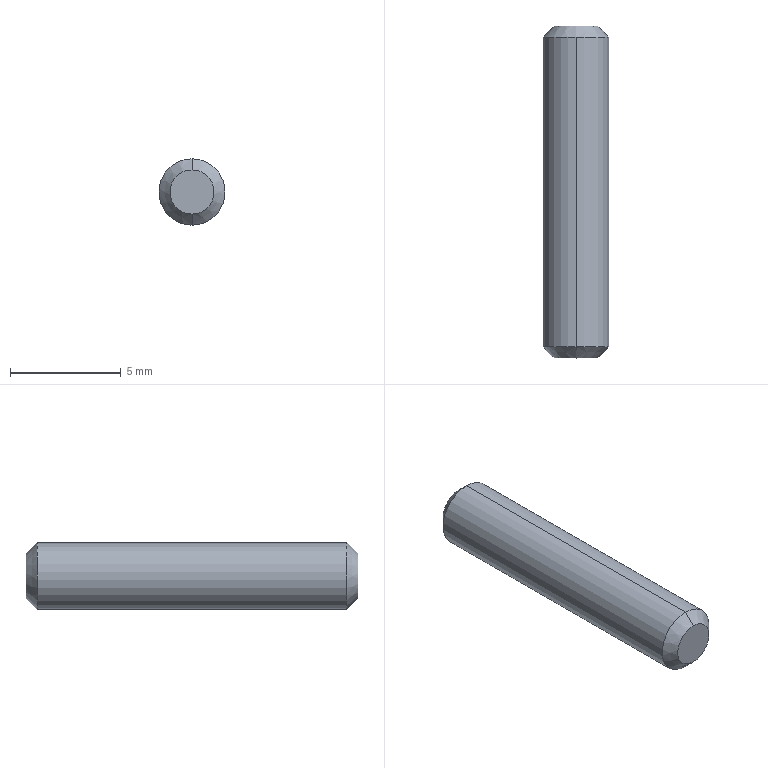Part | SolidWorks | features Chamfer 1, Extrusion 1 | 1 solid | 8 faces | box 3 x 15 x 3 mm | volume 103.934 mm3 | cone 4 | cylinder 2 | plane 2 | commonest cylinder face diameters 3 x2
STEP:
#1=CARTESIAN_POINT('',(0.,15.,1.));
#2=VERTEX_POINT('',#1);
#3=CARTESIAN_POINT('',(0.,15.,-1.));
#4=VERTEX_POINT('',#3);
#5=CARTESIAN_POINT('',(0.,15.,0.));
#6=DIRECTION('',(0.,1.,0.));
#7=DIRECTION('',(0.,0.,1.));
#8=AXIS2_PLACEMENT_3D('',#5,#6,#7);
#9=CIRCLE('',#8,1.);
#10=EDGE_CURVE('',#2,#4,#9,.T.);
#11=ORIENTED_EDGE('',*,*,#10,.F.);
#12=CARTESIAN_POINT('',(0.,14.5,1.5));
#13=VERTEX_POINT('',#12);
#14=CARTESIAN_POINT('',(0.,15.,1.));
#15=DIRECTION('',(0.,-0.7071,0.7071));
#16=VECTOR('',#15,1000.);
#17=LINE('',#14,#16);
#18=EDGE_CURVE('',#2,#13,#17,.T.);
#19=ORIENTED_EDGE('',*,*,#18,.T.);
#20=CARTESIAN_POINT('',(0.,14.5,-1.5));
#21=VERTEX_POINT('',#20);
#22=CARTESIAN_POINT('',(0.,14.5,0.));
#23=DIRECTION('',(0.,-1.,0.));
#24=DIRECTION('',(0.,0.,1.));
#25=AXIS2_PLACEMENT_3D('',#22,#23,#24);
#26=CIRCLE('',#25,1.5);
#27=EDGE_CURVE('',#21,#13,#26,.T.);
#28=ORIENTED_EDGE('',*,*,#27,.F.);
#29=CARTESIAN_POINT('',(0.,15.,-1.));
#30=DIRECTION('',(0.,-0.7071,-0.7071));
#31=VECTOR('',#30,1000.);
#32=LINE('',#29,#31);
#33=EDGE_CURVE('',#4,#21,#32,.T.);
#34=ORIENTED_EDGE('',*,*,#33,.F.);
#35=EDGE_LOOP('',(#11,#19,#28,#34));
#36=FACE_OUTER_BOUND('',#35,.T.);
#37=CARTESIAN_POINT('',(0.,15.,0.));
#38=DIRECTION('',(0.,-1.,0.));
#39=DIRECTION('',(0.,0.,-1.));
#40=AXIS2_PLACEMENT_3D('',#37,#38,#39);
#41=CONICAL_SURFACE('',#40,1.,0.7854);
#42=ADVANCED_FACE('',(#36),#41,.T.);
#43=CARTESIAN_POINT('',(0.,0.,-1.));
#44=VERTEX_POINT('',#43);
#45=CARTESIAN_POINT('',(0.,0.,1.));
#46=VERTEX_POINT('',#45);
#47=CARTESIAN_POINT('',(0.,0.,0.));
#48=DIRECTION('',(0.,-1.,0.));
#49=DIRECTION('',(0.,0.,1.));
#50=AXIS2_PLACEMENT_3D('',#47,#48,#49);
#51=CIRCLE('',#50,1.);
#52=EDGE_CURVE('',#44,#46,#51,.T.);
#53=ORIENTED_EDGE('',*,*,#52,.F.);
#54=CARTESIAN_POINT('',(0.,0.5,-1.5));
#55=VERTEX_POINT('',#54);
#56=CARTESIAN_POINT('',(0.,0.5,-1.5));
#57=DIRECTION('',(0.,0.7071,-0.7071));
#58=VECTOR('',#57,1000.);
#59=LINE('',#56,#58);
#60=EDGE_CURVE('',#44,#55,#59,.T.);
#61=ORIENTED_EDGE('',*,*,#60,.T.);
#62=CARTESIAN_POINT('',(0.,0.5,1.5));
#63=VERTEX_POINT('',#62);
#64=CARTESIAN_POINT('',(0.,0.5,0.));
#65=DIRECTION('',(0.,1.,0.));
#66=DIRECTION('',(0.,0.,1.));
#67=AXIS2_PLACEMENT_3D('',#64,#65,#66);
#68=CIRCLE('',#67,1.5);
#69=EDGE_CURVE('',#63,#55,#68,.T.);
#70=ORIENTED_EDGE('',*,*,#69,.F.);
#71=CARTESIAN_POINT('',(0.,0.5,1.5));
#72=DIRECTION('',(0.,0.7071,0.7071));
#73=VECTOR('',#72,1000.);
#74=LINE('',#71,#73);
#75=EDGE_CURVE('',#46,#63,#74,.T.);
#76=ORIENTED_EDGE('',*,*,#75,.F.);
#77=EDGE_LOOP('',(#53,#61,#70,#76));
#78=FACE_OUTER_BOUND('',#77,.T.);
#79=CARTESIAN_POINT('',(0.,0.5,0.));
#80=DIRECTION('',(0.,1.,0.));
#81=DIRECTION('',(0.,0.,1.));
#82=AXIS2_PLACEMENT_3D('',#79,#80,#81);
#83=CONICAL_SURFACE('',#82,1.5,0.7854);
#84=ADVANCED_FACE('',(#78),#83,.T.);
#85=ORIENTED_EDGE('',*,*,#27,.T.);
#86=CARTESIAN_POINT('',(0.,15.,1.5));
#87=DIRECTION('',(0.,-1.,0.));
#88=VECTOR('',#87,1000.);
#89=LINE('',#86,#88);
#90=EDGE_CURVE('',#13,#63,#89,.T.);
#91=ORIENTED_EDGE('',*,*,#90,.T.);
#92=ORIENTED_EDGE('',*,*,#69,.T.);
#93=CARTESIAN_POINT('',(0.,15.,-1.5));
#94=DIRECTION('',(0.,-1.,0.));
#95=VECTOR('',#94,1000.);
#96=LINE('',#93,#95);
#97=EDGE_CURVE('',#21,#55,#96,.T.);
#98=ORIENTED_EDGE('',*,*,#97,.F.);
#99=EDGE_LOOP('',(#85,#91,#92,#98));
#100=FACE_OUTER_BOUND('',#99,.T.);
#101=CARTESIAN_POINT('',(0.,15.,0.));
#102=DIRECTION('',(0.,-1.,0.));
#103=DIRECTION('',(0.,0.,-1.));
#104=AXIS2_PLACEMENT_3D('',#101,#102,#103);
#105=CYLINDRICAL_SURFACE('',#104,1.5);
#106=ADVANCED_FACE('',(#100),#105,.T.);
#107=ORIENTED_EDGE('',*,*,#90,.F.);
#108=CARTESIAN_POINT('',(0.,14.5,0.));
#109=DIRECTION('',(0.,-1.,0.));
#110=DIRECTION('',(0.,0.,1.));
#111=AXIS2_PLACEMENT_3D('',#108,#109,#110);
#112=CIRCLE('',#111,1.5);
#113=EDGE_CURVE('',#13,#21,#112,.T.);
#114=ORIENTED_EDGE('',*,*,#113,.T.);
#115=ORIENTED_EDGE('',*,*,#97,.T.);
#116=CARTESIAN_POINT('',(0.,0.5,0.));
#117=DIRECTION('',(0.,1.,0.));
#118=DIRECTION('',(0.,0.,1.));
#119=AXIS2_PLACEMENT_3D('',#116,#117,#118);
#120=CIRCLE('',#119,1.5);
#121=EDGE_CURVE('',#55,#63,#120,.T.);
#122=ORIENTED_EDGE('',*,*,#121,.T.);
#123=EDGE_LOOP('',(#107,#114,#115,#122));
#124=FACE_OUTER_BOUND('',#123,.T.);
#125=CARTESIAN_POINT('',(0.,15.,0.));
#126=DIRECTION('',(0.,-1.,0.));
#127=DIRECTION('',(0.,0.,-1.));
#128=AXIS2_PLACEMENT_3D('',#125,#126,#127);
#129=CYLINDRICAL_SURFACE('',#128,1.5);
#130=ADVANCED_FACE('',(#124),#129,.T.);
#131=CARTESIAN_POINT('',(0.,15.,0.));
#132=DIRECTION('',(0.,1.,0.));
#133=DIRECTION('',(0.,0.,1.));
#134=AXIS2_PLACEMENT_3D('',#131,#132,#133);
#135=CIRCLE('',#134,1.);
#136=EDGE_CURVE('',#4,#2,#135,.T.);
#137=ORIENTED_EDGE('',*,*,#136,.T.);
#138=ORIENTED_EDGE('',*,*,#10,.T.);
#139=EDGE_LOOP('',(#137,#138));
#140=FACE_OUTER_BOUND('',#139,.T.);
#141=CARTESIAN_POINT('',(0.,15.,0.));
#142=DIRECTION('',(0.,1.,0.));
#143=DIRECTION('',(0.,0.,1.));
#144=AXIS2_PLACEMENT_3D('',#141,#142,#143);
#145=PLANE('',#144);
#146=ADVANCED_FACE('',(#140),#145,.T.);
#147=CARTESIAN_POINT('',(0.,0.,0.));
#148=DIRECTION('',(0.,-1.,0.));
#149=DIRECTION('',(0.,0.,1.));
#150=AXIS2_PLACEMENT_3D('',#147,#148,#149);
#151=CIRCLE('',#150,1.);
#152=EDGE_CURVE('',#46,#44,#151,.T.);
#153=ORIENTED_EDGE('',*,*,#152,.T.);
#154=ORIENTED_EDGE('',*,*,#52,.T.);
#155=EDGE_LOOP('',(#153,#154));
#156=FACE_OUTER_BOUND('',#155,.T.);
#157=CARTESIAN_POINT('',(0.,0.,0.));
#158=DIRECTION('',(0.,1.,0.));
#159=DIRECTION('',(0.,0.,1.));
#160=AXIS2_PLACEMENT_3D('',#157,#158,#159);
#161=PLANE('',#160);
#162=ADVANCED_FACE('',(#156),#161,.F.);
#163=ORIENTED_EDGE('',*,*,#60,.F.);
#164=ORIENTED_EDGE('',*,*,#152,.F.);
#165=ORIENTED_EDGE('',*,*,#75,.T.);
#166=ORIENTED_EDGE('',*,*,#121,.F.);
#167=EDGE_LOOP('',(#163,#164,#165,#166));
#168=FACE_OUTER_BOUND('',#167,.T.);
#169=CARTESIAN_POINT('',(0.,0.5,0.));
#170=DIRECTION('',(0.,1.,0.));
#171=DIRECTION('',(0.,0.,1.));
#172=AXIS2_PLACEMENT_3D('',#169,#170,#171);
#173=CONICAL_SURFACE('',#172,1.5,0.7854);
#174=ADVANCED_FACE('',(#168),#173,.T.);
#175=ORIENTED_EDGE('',*,*,#18,.F.);
#176=ORIENTED_EDGE('',*,*,#136,.F.);
#177=ORIENTED_EDGE('',*,*,#33,.T.);
#178=ORIENTED_EDGE('',*,*,#113,.F.);
#179=EDGE_LOOP('',(#175,#176,#177,#178));
#180=FACE_OUTER_BOUND('',#179,.T.);
#181=CARTESIAN_POINT('',(0.,15.,0.));
#182=DIRECTION('',(0.,-1.,0.));
#183=DIRECTION('',(0.,0.,-1.));
#184=AXIS2_PLACEMENT_3D('',#181,#182,#183);
#185=CONICAL_SURFACE('',#184,1.,0.7854);
#186=ADVANCED_FACE('',(#180),#185,.T.);
#187=CLOSED_SHELL('',(#42,#84,#106,#130,#146,#162,#174,#186));
#188=MANIFOLD_SOLID_BREP('',#187);
#189=CARTESIAN_POINT('',(0.,0.,0.));
#190=DIRECTION('',(0.,0.,1.));
#191=DIRECTION('',(1.,0.,0.));
#192=AXIS2_PLACEMENT_3D('',#189,#190,#191);
#193=(LENGTH_UNIT()NAMED_UNIT(*)SI_UNIT(.MILLI.,.METRE.));
#194=UNCERTAINTY_MEASURE_WITH_UNIT(LENGTH_MEASURE(0.00001),#193,'','');
#195=(NAMED_UNIT(*)PLANE_ANGLE_UNIT()SI_UNIT($,.RADIAN.));
#196=(NAMED_UNIT(*)SI_UNIT($,.STERADIAN.)SOLID_ANGLE_UNIT());
#197=(GEOMETRIC_REPRESENTATION_CONTEXT(3)GLOBAL_UNCERTAINTY_ASSIGNED_CONTEXT((#194))GLOBAL_UNIT_ASSIGNED_CONTEXT((#193,#195,#196))REPRESENTATION_CONTEXT('',''));
#198=ADVANCED_BREP_SHAPE_REPRESENTATION('',(#188,#192),#197);